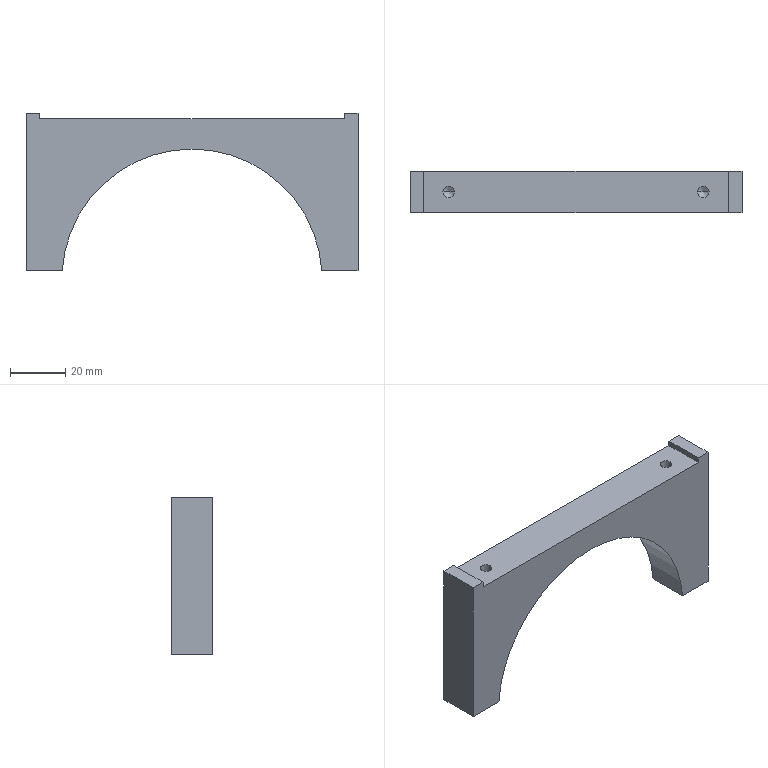Part | STEP file | 11-FG-S01211 | 1 solid | 28 faces | box 120 x 15 x 57 mm | volume 50768 mm3 | plane 11 | cylinder 9 | cone 8 | commonest cylinder face diameters 4.2 x8 94 x1
STEP:
#1=CARTESIAN_POINT('',(-108.1,7.5,42.6));
#2=VERTEX_POINT('',#1);
#3=CARTESIAN_POINT('',(-103.9,7.5,42.6));
#4=VERTEX_POINT('',#3);
#5=CARTESIAN_POINT('',(-106.,7.5,42.6));
#6=DIRECTION('',(0.,0.,1.));
#7=DIRECTION('',(1.,0.,0.));
#8=AXIS2_PLACEMENT_3D('',#5,#6,#7);
#9=CIRCLE('',#8,2.1);
#10=EDGE_CURVE('',#2,#4,#9,.T.);
#11=ORIENTED_EDGE('',*,*,#10,.F.);
#12=CARTESIAN_POINT('',(-108.1,7.5,55.));
#13=VERTEX_POINT('',#12);
#14=CARTESIAN_POINT('',(-108.1,7.5,55.));
#15=DIRECTION('',(0.,0.,1.));
#16=VECTOR('',#15,1000.);
#17=LINE('',#14,#16);
#18=EDGE_CURVE('',#2,#13,#17,.T.);
#19=ORIENTED_EDGE('',*,*,#18,.T.);
#20=CARTESIAN_POINT('',(-103.9,7.5,55.));
#21=VERTEX_POINT('',#20);
#22=CARTESIAN_POINT('',(-106.,7.5,55.));
#23=DIRECTION('',(0.,0.,1.));
#24=DIRECTION('',(1.,0.,0.));
#25=AXIS2_PLACEMENT_3D('',#22,#23,#24);
#26=CIRCLE('',#25,2.1);
#27=EDGE_CURVE('',#13,#21,#26,.T.);
#28=ORIENTED_EDGE('',*,*,#27,.T.);
#29=CARTESIAN_POINT('',(-103.9,7.5,55.));
#30=DIRECTION('',(0.,0.,1.));
#31=VECTOR('',#30,1000.);
#32=LINE('',#29,#31);
#33=EDGE_CURVE('',#4,#21,#32,.T.);
#34=ORIENTED_EDGE('',*,*,#33,.F.);
#35=EDGE_LOOP('',(#11,#19,#28,#34));
#36=FACE_OUTER_BOUND('',#35,.T.);
#37=CARTESIAN_POINT('',(-106.,7.5,55.));
#38=DIRECTION('',(0.,0.,1.));
#39=DIRECTION('',(1.,0.,0.));
#40=AXIS2_PLACEMENT_3D('',#37,#38,#39);
#41=CYLINDRICAL_SURFACE('',#40,2.1);
#42=ADVANCED_FACE('',(#36),#41,.F.);
#43=CARTESIAN_POINT('',(-106.,7.5,41.338));
#44=VERTEX_POINT('',#43);
#45=CARTESIAN_POINT('',(-103.9,7.5,42.6));
#46=DIRECTION('',(0.8572,0.,0.515));
#47=VECTOR('',#46,1000.);
#48=LINE('',#45,#47);
#49=EDGE_CURVE('',#44,#4,#48,.T.);
#50=ORIENTED_EDGE('',*,*,#49,.F.);
#51=CARTESIAN_POINT('',(-108.1,7.5,42.6));
#52=DIRECTION('',(-0.8572,0.,0.515));
#53=VECTOR('',#52,1000.);
#54=LINE('',#51,#53);
#55=EDGE_CURVE('',#44,#2,#54,.T.);
#56=ORIENTED_EDGE('',*,*,#55,.T.);
#57=ORIENTED_EDGE('',*,*,#10,.T.);
#58=EDGE_LOOP('',(#50,#56,#57));
#59=FACE_OUTER_BOUND('',#58,.T.);
#60=CARTESIAN_POINT('',(-106.,7.5,42.6));
#61=DIRECTION('',(0.,0.,1.));
#62=DIRECTION('',(1.,0.,0.));
#63=AXIS2_PLACEMENT_3D('',#60,#61,#62);
#64=CONICAL_SURFACE('',#63,2.1,1.03);
#65=ADVANCED_FACE('',(#59),#64,.F.);
#66=CARTESIAN_POINT('',(-16.1,7.5,42.6));
#67=VERTEX_POINT('',#66);
#68=CARTESIAN_POINT('',(-11.9,7.5,42.6));
#69=VERTEX_POINT('',#68);
#70=CARTESIAN_POINT('',(-14.,7.5,42.6));
#71=DIRECTION('',(0.,0.,1.));
#72=DIRECTION('',(1.,0.,0.));
#73=AXIS2_PLACEMENT_3D('',#70,#71,#72);
#74=CIRCLE('',#73,2.1);
#75=EDGE_CURVE('',#67,#69,#74,.T.);
#76=ORIENTED_EDGE('',*,*,#75,.F.);
#77=CARTESIAN_POINT('',(-16.1,7.5,55.));
#78=VERTEX_POINT('',#77);
#79=CARTESIAN_POINT('',(-16.1,7.5,55.));
#80=DIRECTION('',(0.,0.,1.));
#81=VECTOR('',#80,1000.);
#82=LINE('',#79,#81);
#83=EDGE_CURVE('',#67,#78,#82,.T.);
#84=ORIENTED_EDGE('',*,*,#83,.T.);
#85=CARTESIAN_POINT('',(-11.9,7.5,55.));
#86=VERTEX_POINT('',#85);
#87=CARTESIAN_POINT('',(-14.,7.5,55.));
#88=DIRECTION('',(0.,0.,1.));
#89=DIRECTION('',(1.,0.,0.));
#90=AXIS2_PLACEMENT_3D('',#87,#88,#89);
#91=CIRCLE('',#90,2.1);
#92=EDGE_CURVE('',#78,#86,#91,.T.);
#93=ORIENTED_EDGE('',*,*,#92,.T.);
#94=CARTESIAN_POINT('',(-11.9,7.5,55.));
#95=DIRECTION('',(0.,0.,1.));
#96=VECTOR('',#95,1000.);
#97=LINE('',#94,#96);
#98=EDGE_CURVE('',#69,#86,#97,.T.);
#99=ORIENTED_EDGE('',*,*,#98,.F.);
#100=EDGE_LOOP('',(#76,#84,#93,#99));
#101=FACE_OUTER_BOUND('',#100,.T.);
#102=CARTESIAN_POINT('',(-14.,7.5,55.));
#103=DIRECTION('',(0.,0.,1.));
#104=DIRECTION('',(1.,0.,0.));
#105=AXIS2_PLACEMENT_3D('',#102,#103,#104);
#106=CYLINDRICAL_SURFACE('',#105,2.1);
#107=ADVANCED_FACE('',(#101),#106,.F.);
#108=CARTESIAN_POINT('',(-14.,7.5,41.338));
#109=VERTEX_POINT('',#108);
#110=CARTESIAN_POINT('',(-11.9,7.5,42.6));
#111=DIRECTION('',(0.8572,0.,0.515));
#112=VECTOR('',#111,1000.);
#113=LINE('',#110,#112);
#114=EDGE_CURVE('',#109,#69,#113,.T.);
#115=ORIENTED_EDGE('',*,*,#114,.F.);
#116=CARTESIAN_POINT('',(-16.1,7.5,42.6));
#117=DIRECTION('',(-0.8572,0.,0.515));
#118=VECTOR('',#117,1000.);
#119=LINE('',#116,#118);
#120=EDGE_CURVE('',#109,#67,#119,.T.);
#121=ORIENTED_EDGE('',*,*,#120,.T.);
#122=ORIENTED_EDGE('',*,*,#75,.T.);
#123=EDGE_LOOP('',(#115,#121,#122));
#124=FACE_OUTER_BOUND('',#123,.T.);
#125=CARTESIAN_POINT('',(-14.,7.5,42.6));
#126=DIRECTION('',(0.,0.,1.));
#127=DIRECTION('',(1.,0.,0.));
#128=AXIS2_PLACEMENT_3D('',#125,#126,#127);
#129=CONICAL_SURFACE('',#128,2.1,1.03);
#130=ADVANCED_FACE('',(#124),#129,.F.);
#131=CARTESIAN_POINT('',(-111.4,7.5,12.4));
#132=VERTEX_POINT('',#131);
#133=CARTESIAN_POINT('',(-115.6,7.5,12.4));
#134=VERTEX_POINT('',#133);
#135=CARTESIAN_POINT('',(-113.5,7.5,12.4));
#136=DIRECTION('',(0.,0.,-1.));
#137=DIRECTION('',(-1.,0.,0.));
#138=AXIS2_PLACEMENT_3D('',#135,#136,#137);
#139=CIRCLE('',#138,2.1);
#140=EDGE_CURVE('',#132,#134,#139,.T.);
#141=ORIENTED_EDGE('',*,*,#140,.F.);
#142=CARTESIAN_POINT('',(-111.4,7.5,0.));
#143=VERTEX_POINT('',#142);
#144=CARTESIAN_POINT('',(-111.4,7.5,0.));
#145=DIRECTION('',(0.,0.,-1.));
#146=VECTOR('',#145,1000.);
#147=LINE('',#144,#146);
#148=EDGE_CURVE('',#132,#143,#147,.T.);
#149=ORIENTED_EDGE('',*,*,#148,.T.);
#150=CARTESIAN_POINT('',(-115.6,7.5,0.));
#151=VERTEX_POINT('',#150);
#152=CARTESIAN_POINT('',(-113.5,7.5,0.));
#153=DIRECTION('',(0.,0.,-1.));
#154=DIRECTION('',(-1.,0.,0.));
#155=AXIS2_PLACEMENT_3D('',#152,#153,#154);
#156=CIRCLE('',#155,2.1);
#157=EDGE_CURVE('',#143,#151,#156,.T.);
#158=ORIENTED_EDGE('',*,*,#157,.T.);
#159=CARTESIAN_POINT('',(-115.6,7.5,0.));
#160=DIRECTION('',(0.,0.,-1.));
#161=VECTOR('',#160,1000.);
#162=LINE('',#159,#161);
#163=EDGE_CURVE('',#134,#151,#162,.T.);
#164=ORIENTED_EDGE('',*,*,#163,.F.);
#165=EDGE_LOOP('',(#141,#149,#158,#164));
#166=FACE_OUTER_BOUND('',#165,.T.);
#167=CARTESIAN_POINT('',(-113.5,7.5,0.));
#168=DIRECTION('',(0.,0.,-1.));
#169=DIRECTION('',(-1.,0.,0.));
#170=AXIS2_PLACEMENT_3D('',#167,#168,#169);
#171=CYLINDRICAL_SURFACE('',#170,2.1);
#172=ADVANCED_FACE('',(#166),#171,.F.);
#173=CARTESIAN_POINT('',(-113.5,7.5,13.662));
#174=VERTEX_POINT('',#173);
#175=CARTESIAN_POINT('',(-115.6,7.5,12.4));
#176=DIRECTION('',(-0.8572,0.,-0.515));
#177=VECTOR('',#176,1000.);
#178=LINE('',#175,#177);
#179=EDGE_CURVE('',#174,#134,#178,.T.);
#180=ORIENTED_EDGE('',*,*,#179,.F.);
#181=CARTESIAN_POINT('',(-111.4,7.5,12.4));
#182=DIRECTION('',(0.8572,0.,-0.515));
#183=VECTOR('',#182,1000.);
#184=LINE('',#181,#183);
#185=EDGE_CURVE('',#174,#132,#184,.T.);
#186=ORIENTED_EDGE('',*,*,#185,.T.);
#187=ORIENTED_EDGE('',*,*,#140,.T.);
#188=EDGE_LOOP('',(#180,#186,#187));
#189=FACE_OUTER_BOUND('',#188,.T.);
#190=CARTESIAN_POINT('',(-113.5,7.5,12.4));
#191=DIRECTION('',(0.,0.,-1.));
#192=DIRECTION('',(-1.,0.,0.));
#193=AXIS2_PLACEMENT_3D('',#190,#191,#192);
#194=CONICAL_SURFACE('',#193,2.1,1.03);
#195=ADVANCED_FACE('',(#189),#194,.F.);
#196=CARTESIAN_POINT('',(-4.4,7.5,12.4));
#197=VERTEX_POINT('',#196);
#198=CARTESIAN_POINT('',(-8.6,7.5,12.4));
#199=VERTEX_POINT('',#198);
#200=CARTESIAN_POINT('',(-6.5,7.5,12.4));
#201=DIRECTION('',(0.,0.,-1.));
#202=DIRECTION('',(-1.,0.,0.));
#203=AXIS2_PLACEMENT_3D('',#200,#201,#202);
#204=CIRCLE('',#203,2.1);
#205=EDGE_CURVE('',#197,#199,#204,.T.);
#206=ORIENTED_EDGE('',*,*,#205,.F.);
#207=CARTESIAN_POINT('',(-4.4,7.5,0.));
#208=VERTEX_POINT('',#207);
#209=CARTESIAN_POINT('',(-4.4,7.5,0.));
#210=DIRECTION('',(0.,0.,-1.));
#211=VECTOR('',#210,1000.);
#212=LINE('',#209,#211);
#213=EDGE_CURVE('',#197,#208,#212,.T.);
#214=ORIENTED_EDGE('',*,*,#213,.T.);
#215=CARTESIAN_POINT('',(-8.6,7.5,0.));
#216=VERTEX_POINT('',#215);
#217=CARTESIAN_POINT('',(-6.5,7.5,0.));
#218=DIRECTION('',(0.,0.,-1.));
#219=DIRECTION('',(-1.,0.,0.));
#220=AXIS2_PLACEMENT_3D('',#217,#218,#219);
#221=CIRCLE('',#220,2.1);
#222=EDGE_CURVE('',#208,#216,#221,.T.);
#223=ORIENTED_EDGE('',*,*,#222,.T.);
#224=CARTESIAN_POINT('',(-8.6,7.5,0.));
#225=DIRECTION('',(0.,0.,-1.));
#226=VECTOR('',#225,1000.);
#227=LINE('',#224,#226);
#228=EDGE_CURVE('',#199,#216,#227,.T.);
#229=ORIENTED_EDGE('',*,*,#228,.F.);
#230=EDGE_LOOP('',(#206,#214,#223,#229));
#231=FACE_OUTER_BOUND('',#230,.T.);
#232=CARTESIAN_POINT('',(-6.5,7.5,0.));
#233=DIRECTION('',(0.,0.,-1.));
#234=DIRECTION('',(-1.,0.,0.));
#235=AXIS2_PLACEMENT_3D('',#232,#233,#234);
#236=CYLINDRICAL_SURFACE('',#235,2.1);
#237=ADVANCED_FACE('',(#231),#236,.F.);
#238=CARTESIAN_POINT('',(-6.5,7.5,13.662));
#239=VERTEX_POINT('',#238);
#240=CARTESIAN_POINT('',(-8.6,7.5,12.4));
#241=DIRECTION('',(-0.8572,0.,-0.515));
#242=VECTOR('',#241,1000.);
#243=LINE('',#240,#242);
#244=EDGE_CURVE('',#239,#199,#243,.T.);
#245=ORIENTED_EDGE('',*,*,#244,.F.);
#246=CARTESIAN_POINT('',(-4.4,7.5,12.4));
#247=DIRECTION('',(0.8572,0.,-0.515));
#248=VECTOR('',#247,1000.);
#249=LINE('',#246,#248);
#250=EDGE_CURVE('',#239,#197,#249,.T.);
#251=ORIENTED_EDGE('',*,*,#250,.T.);
#252=ORIENTED_EDGE('',*,*,#205,.T.);
#253=EDGE_LOOP('',(#245,#251,#252));
#254=FACE_OUTER_BOUND('',#253,.T.);
#255=CARTESIAN_POINT('',(-6.5,7.5,12.4));
#256=DIRECTION('',(0.,0.,-1.));
#257=DIRECTION('',(-1.,0.,0.));
#258=AXIS2_PLACEMENT_3D('',#255,#256,#257);
#259=CONICAL_SURFACE('',#258,2.1,1.03);
#260=ADVANCED_FACE('',(#254),#259,.F.);
#261=CARTESIAN_POINT('',(-120.,0.,57.));
#262=VERTEX_POINT('',#261);
#263=CARTESIAN_POINT('',(-115.,0.,57.));
#264=VERTEX_POINT('',#263);
#265=CARTESIAN_POINT('',(-201.,0.,57.));
#266=DIRECTION('',(1.,0.,0.));
#267=VECTOR('',#266,1000.);
#268=LINE('',#265,#267);
#269=EDGE_CURVE('',#262,#264,#268,.T.);
#270=ORIENTED_EDGE('',*,*,#269,.T.);
#271=CARTESIAN_POINT('',(-115.,15.,57.));
#272=VERTEX_POINT('',#271);
#273=CARTESIAN_POINT('',(-115.,15.,57.));
#274=DIRECTION('',(0.,1.,0.));
#275=VECTOR('',#274,1000.);
#276=LINE('',#273,#275);
#277=EDGE_CURVE('',#264,#272,#276,.T.);
#278=ORIENTED_EDGE('',*,*,#277,.T.);
#279=CARTESIAN_POINT('',(-120.,15.,57.));
#280=VERTEX_POINT('',#279);
#281=CARTESIAN_POINT('',(-201.,15.,57.));
#282=DIRECTION('',(1.,0.,0.));
#283=VECTOR('',#282,1000.);
#284=LINE('',#281,#283);
#285=EDGE_CURVE('',#280,#272,#284,.T.);
#286=ORIENTED_EDGE('',*,*,#285,.F.);
#287=CARTESIAN_POINT('',(-120.,0.,57.));
#288=DIRECTION('',(0.,1.,0.));
#289=VECTOR('',#288,1000.);
#290=LINE('',#287,#289);
#291=EDGE_CURVE('',#262,#280,#290,.T.);
#292=ORIENTED_EDGE('',*,*,#291,.F.);
#293=EDGE_LOOP('',(#270,#278,#286,#292));
#294=FACE_OUTER_BOUND('',#293,.T.);
#295=CARTESIAN_POINT('',(-201.,15.,57.));
#296=DIRECTION('',(0.,0.,-1.));
#297=DIRECTION('',(0.,1.,0.));
#298=AXIS2_PLACEMENT_3D('',#295,#296,#297);
#299=PLANE('',#298);
#300=ADVANCED_FACE('',(#294),#299,.F.);
#301=CARTESIAN_POINT('',(-113.5,7.5,0.));
#302=DIRECTION('',(0.,0.,-1.));
#303=DIRECTION('',(-1.,0.,0.));
#304=AXIS2_PLACEMENT_3D('',#301,#302,#303);
#305=CIRCLE('',#304,2.1);
#306=EDGE_CURVE('',#151,#143,#305,.T.);
#307=ORIENTED_EDGE('',*,*,#306,.F.);
#308=ORIENTED_EDGE('',*,*,#157,.F.);
#309=EDGE_LOOP('',(#307,#308));
#310=FACE_BOUND('',#309,.T.);
#311=CARTESIAN_POINT('',(-106.904,15.,0.));
#312=VERTEX_POINT('',#311);
#313=CARTESIAN_POINT('',(-120.,15.,0.));
#314=VERTEX_POINT('',#313);
#315=CARTESIAN_POINT('',(0.,15.,0.));
#316=DIRECTION('',(-1.,0.,0.));
#317=VECTOR('',#316,1000.);
#318=LINE('',#315,#317);
#319=EDGE_CURVE('',#312,#314,#318,.T.);
#320=ORIENTED_EDGE('',*,*,#319,.F.);
#321=CARTESIAN_POINT('',(-106.904,0.,0.));
#322=VERTEX_POINT('',#321);
#323=CARTESIAN_POINT('',(-106.904,80.,0.));
#324=DIRECTION('',(0.,-1.,0.));
#325=VECTOR('',#324,1000.);
#326=LINE('',#323,#325);
#327=EDGE_CURVE('',#312,#322,#326,.T.);
#328=ORIENTED_EDGE('',*,*,#327,.T.);
#329=CARTESIAN_POINT('',(-120.,0.,0.));
#330=VERTEX_POINT('',#329);
#331=CARTESIAN_POINT('',(0.,0.,0.));
#332=DIRECTION('',(1.,0.,0.));
#333=VECTOR('',#332,1000.);
#334=LINE('',#331,#333);
#335=EDGE_CURVE('',#330,#322,#334,.T.);
#336=ORIENTED_EDGE('',*,*,#335,.F.);
#337=CARTESIAN_POINT('',(-120.,0.,0.));
#338=DIRECTION('',(0.,-1.,0.));
#339=VECTOR('',#338,1000.);
#340=LINE('',#337,#339);
#341=EDGE_CURVE('',#314,#330,#340,.T.);
#342=ORIENTED_EDGE('',*,*,#341,.F.);
#343=EDGE_LOOP('',(#320,#328,#336,#342));
#344=FACE_OUTER_BOUND('',#343,.T.);
#345=CARTESIAN_POINT('',(0.,15.,0.));
#346=DIRECTION('',(0.,0.,1.));
#347=DIRECTION('',(1.,0.,0.));
#348=AXIS2_PLACEMENT_3D('',#345,#346,#347);
#349=PLANE('',#348);
#350=ADVANCED_FACE('',(#310,#344),#349,.F.);
#351=CARTESIAN_POINT('',(0.,15.,57.));
#352=VERTEX_POINT('',#351);
#353=CARTESIAN_POINT('',(0.,15.,0.));
#354=VERTEX_POINT('',#353);
#355=CARTESIAN_POINT('',(0.,15.,60.));
#356=DIRECTION('',(0.,0.,-1.));
#357=VECTOR('',#356,1000.);
#358=LINE('',#355,#357);
#359=EDGE_CURVE('',#352,#354,#358,.T.);
#360=ORIENTED_EDGE('',*,*,#359,.F.);
#361=CARTESIAN_POINT('',(0.,0.,57.));
#362=VERTEX_POINT('',#361);
#363=CARTESIAN_POINT('',(0.,15.,57.));
#364=DIRECTION('',(0.,1.,0.));
#365=VECTOR('',#364,1000.);
#366=LINE('',#363,#365);
#367=EDGE_CURVE('',#362,#352,#366,.T.);
#368=ORIENTED_EDGE('',*,*,#367,.F.);
#369=CARTESIAN_POINT('',(0.,0.,0.));
#370=VERTEX_POINT('',#369);
#371=CARTESIAN_POINT('',(0.,0.,60.));
#372=DIRECTION('',(0.,0.,-1.));
#373=VECTOR('',#372,1000.);
#374=LINE('',#371,#373);
#375=EDGE_CURVE('',#362,#370,#374,.T.);
#376=ORIENTED_EDGE('',*,*,#375,.T.);
#377=CARTESIAN_POINT('',(0.,0.,0.));
#378=DIRECTION('',(0.,1.,0.));
#379=VECTOR('',#378,1000.);
#380=LINE('',#377,#379);
#381=EDGE_CURVE('',#370,#354,#380,.T.);
#382=ORIENTED_EDGE('',*,*,#381,.T.);
#383=EDGE_LOOP('',(#360,#368,#376,#382));
#384=FACE_OUTER_BOUND('',#383,.T.);
#385=CARTESIAN_POINT('',(0.,0.,60.));
#386=DIRECTION('',(-1.,0.,0.));
#387=DIRECTION('',(0.,0.,1.));
#388=AXIS2_PLACEMENT_3D('',#385,#386,#387);
#389=PLANE('',#388);
#390=ADVANCED_FACE('',(#384),#389,.F.);
#391=ORIENTED_EDGE('',*,*,#285,.T.);
#392=CARTESIAN_POINT('',(-115.,15.,55.));
#393=VERTEX_POINT('',#392);
#394=CARTESIAN_POINT('',(-115.,15.,57.));
#395=DIRECTION('',(0.,0.,1.));
#396=VECTOR('',#395,1000.);
#397=LINE('',#394,#396);
#398=EDGE_CURVE('',#393,#272,#397,.T.);
#399=ORIENTED_EDGE('',*,*,#398,.F.);
#400=CARTESIAN_POINT('',(-5.,15.,55.));
#401=VERTEX_POINT('',#400);
#402=CARTESIAN_POINT('',(-115.,15.,55.));
#403=DIRECTION('',(-1.,0.,0.));
#404=VECTOR('',#403,1000.);
#405=LINE('',#402,#404);
#406=EDGE_CURVE('',#401,#393,#405,.T.);
#407=ORIENTED_EDGE('',*,*,#406,.F.);
#408=CARTESIAN_POINT('',(-5.,15.,57.));
#409=VERTEX_POINT('',#408);
#410=CARTESIAN_POINT('',(-5.,15.,57.));
#411=DIRECTION('',(0.,0.,-1.));
#412=VECTOR('',#411,1000.);
#413=LINE('',#410,#412);
#414=EDGE_CURVE('',#409,#401,#413,.T.);
#415=ORIENTED_EDGE('',*,*,#414,.F.);
#416=CARTESIAN_POINT('',(-201.,15.,57.));
#417=DIRECTION('',(1.,0.,0.));
#418=VECTOR('',#417,1000.);
#419=LINE('',#416,#418);
#420=EDGE_CURVE('',#409,#352,#419,.T.);
#421=ORIENTED_EDGE('',*,*,#420,.T.);
#422=ORIENTED_EDGE('',*,*,#359,.T.);
#423=CARTESIAN_POINT('',(-13.096,15.,0.));
#424=VERTEX_POINT('',#423);
#425=CARTESIAN_POINT('',(0.,15.,0.));
#426=DIRECTION('',(-1.,0.,0.));
#427=VECTOR('',#426,1000.);
#428=LINE('',#425,#427);
#429=EDGE_CURVE('',#354,#424,#428,.T.);
#430=ORIENTED_EDGE('',*,*,#429,.T.);
#431=CARTESIAN_POINT('',(-60.,15.,-3.));
#432=DIRECTION('',(0.,-1.,0.));
#433=DIRECTION('',(1.,0.,0.));
#434=AXIS2_PLACEMENT_3D('',#431,#432,#433);
#435=CIRCLE('',#434,47.);
#436=EDGE_CURVE('',#424,#312,#435,.T.);
#437=ORIENTED_EDGE('',*,*,#436,.T.);
#438=ORIENTED_EDGE('',*,*,#319,.T.);
#439=CARTESIAN_POINT('',(-120.,15.,60.));
#440=DIRECTION('',(0.,0.,-1.));
#441=VECTOR('',#440,1000.);
#442=LINE('',#439,#441);
#443=EDGE_CURVE('',#280,#314,#442,.T.);
#444=ORIENTED_EDGE('',*,*,#443,.F.);
#445=EDGE_LOOP('',(#391,#399,#407,#415,#421,#422,#430,#437,#438,#444));
#446=FACE_OUTER_BOUND('',#445,.T.);
#447=CARTESIAN_POINT('',(0.,15.,60.));
#448=DIRECTION('',(0.,-1.,0.));
#449=DIRECTION('',(1.,0.,0.));
#450=AXIS2_PLACEMENT_3D('',#447,#448,#449);
#451=PLANE('',#450);
#452=ADVANCED_FACE('',(#446),#451,.F.);
#453=CARTESIAN_POINT('',(-120.,0.,60.));
#454=DIRECTION('',(0.,0.,-1.));
#455=VECTOR('',#454,1000.);
#456=LINE('',#453,#455);
#457=EDGE_CURVE('',#262,#330,#456,.T.);
#458=ORIENTED_EDGE('',*,*,#457,.F.);
#459=ORIENTED_EDGE('',*,*,#291,.T.);
#460=ORIENTED_EDGE('',*,*,#443,.T.);
#461=ORIENTED_EDGE('',*,*,#341,.T.);
#462=EDGE_LOOP('',(#458,#459,#460,#461));
#463=FACE_OUTER_BOUND('',#462,.T.);
#464=CARTESIAN_POINT('',(-120.,0.,60.));
#465=DIRECTION('',(1.,0.,0.));
#466=DIRECTION('',(0.,0.,-1.));
#467=AXIS2_PLACEMENT_3D('',#464,#465,#466);
#468=PLANE('',#467);
#469=ADVANCED_FACE('',(#463),#468,.F.);
#470=CARTESIAN_POINT('',(-5.,0.,55.));
#471=VERTEX_POINT('',#470);
#472=CARTESIAN_POINT('',(-115.,0.,55.));
#473=VERTEX_POINT('',#472);
#474=CARTESIAN_POINT('',(0.,0.,55.));
#475=DIRECTION('',(-1.,0.,0.));
#476=VECTOR('',#475,1000.);
#477=LINE('',#474,#476);
#478=EDGE_CURVE('',#471,#473,#477,.T.);
#479=ORIENTED_EDGE('',*,*,#478,.T.);
#480=CARTESIAN_POINT('',(-115.,0.,60.));
#481=DIRECTION('',(0.,0.,1.));
#482=VECTOR('',#481,1000.);
#483=LINE('',#480,#482);
#484=EDGE_CURVE('',#473,#264,#483,.T.);
#485=ORIENTED_EDGE('',*,*,#484,.T.);
#486=ORIENTED_EDGE('',*,*,#269,.F.);
#487=ORIENTED_EDGE('',*,*,#457,.T.);
#488=ORIENTED_EDGE('',*,*,#335,.T.);
#489=CARTESIAN_POINT('',(-13.096,0.,0.));
#490=VERTEX_POINT('',#489);
#491=CARTESIAN_POINT('',(-60.,0.,-3.));
#492=DIRECTION('',(0.,-1.,0.));
#493=DIRECTION('',(1.,0.,0.));
#494=AXIS2_PLACEMENT_3D('',#491,#492,#493);
#495=CIRCLE('',#494,47.);
#496=EDGE_CURVE('',#490,#322,#495,.T.);
#497=ORIENTED_EDGE('',*,*,#496,.F.);
#498=CARTESIAN_POINT('',(0.,0.,0.));
#499=DIRECTION('',(1.,0.,0.));
#500=VECTOR('',#499,1000.);
#501=LINE('',#498,#500);
#502=EDGE_CURVE('',#490,#370,#501,.T.);
#503=ORIENTED_EDGE('',*,*,#502,.T.);
#504=ORIENTED_EDGE('',*,*,#375,.F.);
#505=CARTESIAN_POINT('',(-5.,0.,57.));
#506=VERTEX_POINT('',#505);
#507=CARTESIAN_POINT('',(-201.,0.,57.));
#508=DIRECTION('',(1.,0.,0.));
#509=VECTOR('',#508,1000.);
#510=LINE('',#507,#509);
#511=EDGE_CURVE('',#506,#362,#510,.T.);
#512=ORIENTED_EDGE('',*,*,#511,.F.);
#513=CARTESIAN_POINT('',(-5.,0.,60.));
#514=DIRECTION('',(0.,0.,-1.));
#515=VECTOR('',#514,1000.);
#516=LINE('',#513,#515);
#517=EDGE_CURVE('',#506,#471,#516,.T.);
#518=ORIENTED_EDGE('',*,*,#517,.T.);
#519=EDGE_LOOP('',(#479,#485,#486,#487,#488,#497,#503,#504,#512,#518));
#520=FACE_OUTER_BOUND('',#519,.T.);
#521=CARTESIAN_POINT('',(0.,0.,60.));
#522=DIRECTION('',(0.,1.,0.));
#523=DIRECTION('',(-1.,0.,0.));
#524=AXIS2_PLACEMENT_3D('',#521,#522,#523);
#525=PLANE('',#524);
#526=ADVANCED_FACE('',(#520),#525,.F.);
#527=CARTESIAN_POINT('',(-6.5,7.5,0.));
#528=DIRECTION('',(0.,0.,-1.));
#529=DIRECTION('',(-1.,0.,0.));
#530=AXIS2_PLACEMENT_3D('',#527,#528,#529);
#531=CIRCLE('',#530,2.1);
#532=EDGE_CURVE('',#216,#208,#531,.T.);
#533=ORIENTED_EDGE('',*,*,#532,.F.);
#534=ORIENTED_EDGE('',*,*,#222,.F.);
#535=EDGE_LOOP('',(#533,#534));
#536=FACE_BOUND('',#535,.T.);
#537=ORIENTED_EDGE('',*,*,#502,.F.);
#538=CARTESIAN_POINT('',(-13.096,80.,0.));
#539=DIRECTION('',(0.,1.,0.));
#540=VECTOR('',#539,1000.);
#541=LINE('',#538,#540);
#542=EDGE_CURVE('',#490,#424,#541,.T.);
#543=ORIENTED_EDGE('',*,*,#542,.T.);
#544=ORIENTED_EDGE('',*,*,#429,.F.);
#545=ORIENTED_EDGE('',*,*,#381,.F.);
#546=EDGE_LOOP('',(#537,#543,#544,#545));
#547=FACE_OUTER_BOUND('',#546,.T.);
#548=CARTESIAN_POINT('',(0.,15.,0.));
#549=DIRECTION('',(0.,0.,1.));
#550=DIRECTION('',(1.,0.,0.));
#551=AXIS2_PLACEMENT_3D('',#548,#549,#550);
#552=PLANE('',#551);
#553=ADVANCED_FACE('',(#536,#547),#552,.F.);
#554=ORIENTED_EDGE('',*,*,#436,.F.);
#555=ORIENTED_EDGE('',*,*,#542,.F.);
#556=ORIENTED_EDGE('',*,*,#496,.T.);
#557=ORIENTED_EDGE('',*,*,#327,.F.);
#558=EDGE_LOOP('',(#554,#555,#556,#557));
#559=FACE_OUTER_BOUND('',#558,.T.);
#560=CARTESIAN_POINT('',(-60.,80.,-3.));
#561=DIRECTION('',(0.,-1.,0.));
#562=DIRECTION('',(1.,0.,0.));
#563=AXIS2_PLACEMENT_3D('',#560,#561,#562);
#564=CYLINDRICAL_SURFACE('',#563,47.);
#565=ADVANCED_FACE('',(#559),#564,.F.);
#566=ORIENTED_EDGE('',*,*,#250,.F.);
#567=ORIENTED_EDGE('',*,*,#244,.T.);
#568=CARTESIAN_POINT('',(-6.5,7.5,12.4));
#569=DIRECTION('',(0.,0.,-1.));
#570=DIRECTION('',(-1.,0.,0.));
#571=AXIS2_PLACEMENT_3D('',#568,#569,#570);
#572=CIRCLE('',#571,2.1);
#573=EDGE_CURVE('',#199,#197,#572,.T.);
#574=ORIENTED_EDGE('',*,*,#573,.T.);
#575=EDGE_LOOP('',(#566,#567,#574));
#576=FACE_OUTER_BOUND('',#575,.T.);
#577=CARTESIAN_POINT('',(-6.5,7.5,12.4));
#578=DIRECTION('',(0.,0.,-1.));
#579=DIRECTION('',(-1.,0.,0.));
#580=AXIS2_PLACEMENT_3D('',#577,#578,#579);
#581=CONICAL_SURFACE('',#580,2.1,1.03);
#582=ADVANCED_FACE('',(#576),#581,.F.);
#583=ORIENTED_EDGE('',*,*,#213,.F.);
#584=ORIENTED_EDGE('',*,*,#573,.F.);
#585=ORIENTED_EDGE('',*,*,#228,.T.);
#586=ORIENTED_EDGE('',*,*,#532,.T.);
#587=EDGE_LOOP('',(#583,#584,#585,#586));
#588=FACE_OUTER_BOUND('',#587,.T.);
#589=CARTESIAN_POINT('',(-6.5,7.5,0.));
#590=DIRECTION('',(0.,0.,-1.));
#591=DIRECTION('',(-1.,0.,0.));
#592=AXIS2_PLACEMENT_3D('',#589,#590,#591);
#593=CYLINDRICAL_SURFACE('',#592,2.1);
#594=ADVANCED_FACE('',(#588),#593,.F.);
#595=ORIENTED_EDGE('',*,*,#185,.F.);
#596=ORIENTED_EDGE('',*,*,#179,.T.);
#597=CARTESIAN_POINT('',(-113.5,7.5,12.4));
#598=DIRECTION('',(0.,0.,-1.));
#599=DIRECTION('',(-1.,0.,0.));
#600=AXIS2_PLACEMENT_3D('',#597,#598,#599);
#601=CIRCLE('',#600,2.1);
#602=EDGE_CURVE('',#134,#132,#601,.T.);
#603=ORIENTED_EDGE('',*,*,#602,.T.);
#604=EDGE_LOOP('',(#595,#596,#603));
#605=FACE_OUTER_BOUND('',#604,.T.);
#606=CARTESIAN_POINT('',(-113.5,7.5,12.4));
#607=DIRECTION('',(0.,0.,-1.));
#608=DIRECTION('',(-1.,0.,0.));
#609=AXIS2_PLACEMENT_3D('',#606,#607,#608);
#610=CONICAL_SURFACE('',#609,2.1,1.03);
#611=ADVANCED_FACE('',(#605),#610,.F.);
#612=ORIENTED_EDGE('',*,*,#148,.F.);
#613=ORIENTED_EDGE('',*,*,#602,.F.);
#614=ORIENTED_EDGE('',*,*,#163,.T.);
#615=ORIENTED_EDGE('',*,*,#306,.T.);
#616=EDGE_LOOP('',(#612,#613,#614,#615));
#617=FACE_OUTER_BOUND('',#616,.T.);
#618=CARTESIAN_POINT('',(-113.5,7.5,0.));
#619=DIRECTION('',(0.,0.,-1.));
#620=DIRECTION('',(-1.,0.,0.));
#621=AXIS2_PLACEMENT_3D('',#618,#619,#620);
#622=CYLINDRICAL_SURFACE('',#621,2.1);
#623=ADVANCED_FACE('',(#617),#622,.F.);
#624=ORIENTED_EDGE('',*,*,#420,.F.);
#625=CARTESIAN_POINT('',(-5.,15.,57.));
#626=DIRECTION('',(0.,-1.,0.));
#627=VECTOR('',#626,1000.);
#628=LINE('',#625,#627);
#629=EDGE_CURVE('',#409,#506,#628,.T.);
#630=ORIENTED_EDGE('',*,*,#629,.T.);
#631=ORIENTED_EDGE('',*,*,#511,.T.);
#632=ORIENTED_EDGE('',*,*,#367,.T.);
#633=EDGE_LOOP('',(#624,#630,#631,#632));
#634=FACE_OUTER_BOUND('',#633,.T.);
#635=CARTESIAN_POINT('',(-201.,15.,57.));
#636=DIRECTION('',(0.,0.,-1.));
#637=DIRECTION('',(0.,1.,0.));
#638=AXIS2_PLACEMENT_3D('',#635,#636,#637);
#639=PLANE('',#638);
#640=ADVANCED_FACE('',(#634),#639,.F.);
#641=CARTESIAN_POINT('',(-106.,7.5,55.));
#642=DIRECTION('',(0.,0.,1.));
#643=DIRECTION('',(1.,0.,0.));
#644=AXIS2_PLACEMENT_3D('',#641,#642,#643);
#645=CIRCLE('',#644,2.1);
#646=EDGE_CURVE('',#21,#13,#645,.T.);
#647=ORIENTED_EDGE('',*,*,#646,.F.);
#648=ORIENTED_EDGE('',*,*,#27,.F.);
#649=EDGE_LOOP('',(#647,#648));
#650=FACE_BOUND('',#649,.T.);
#651=CARTESIAN_POINT('',(-14.,7.5,55.));
#652=DIRECTION('',(0.,0.,1.));
#653=DIRECTION('',(1.,0.,0.));
#654=AXIS2_PLACEMENT_3D('',#651,#652,#653);
#655=CIRCLE('',#654,2.1);
#656=EDGE_CURVE('',#86,#78,#655,.T.);
#657=ORIENTED_EDGE('',*,*,#656,.F.);
#658=ORIENTED_EDGE('',*,*,#92,.F.);
#659=EDGE_LOOP('',(#657,#658));
#660=FACE_BOUND('',#659,.T.);
#661=CARTESIAN_POINT('',(-5.,-186.,55.));
#662=DIRECTION('',(0.,1.,0.));
#663=VECTOR('',#662,1000.);
#664=LINE('',#661,#663);
#665=EDGE_CURVE('',#471,#401,#664,.T.);
#666=ORIENTED_EDGE('',*,*,#665,.T.);
#667=ORIENTED_EDGE('',*,*,#406,.T.);
#668=CARTESIAN_POINT('',(-115.,-186.,55.));
#669=DIRECTION('',(0.,1.,0.));
#670=VECTOR('',#669,1000.);
#671=LINE('',#668,#670);
#672=EDGE_CURVE('',#473,#393,#671,.T.);
#673=ORIENTED_EDGE('',*,*,#672,.F.);
#674=ORIENTED_EDGE('',*,*,#478,.F.);
#675=EDGE_LOOP('',(#666,#667,#673,#674));
#676=FACE_OUTER_BOUND('',#675,.T.);
#677=CARTESIAN_POINT('',(-115.,-186.,55.));
#678=DIRECTION('',(0.,0.,-1.));
#679=DIRECTION('',(-1.,0.,0.));
#680=AXIS2_PLACEMENT_3D('',#677,#678,#679);
#681=PLANE('',#680);
#682=ADVANCED_FACE('',(#650,#660,#676),#681,.F.);
#683=ORIENTED_EDGE('',*,*,#672,.T.);
#684=ORIENTED_EDGE('',*,*,#398,.T.);
#685=ORIENTED_EDGE('',*,*,#277,.F.);
#686=ORIENTED_EDGE('',*,*,#484,.F.);
#687=EDGE_LOOP('',(#683,#684,#685,#686));
#688=FACE_OUTER_BOUND('',#687,.T.);
#689=CARTESIAN_POINT('',(-115.,-186.,57.));
#690=DIRECTION('',(-1.,0.,0.));
#691=DIRECTION('',(0.,-1.,0.));
#692=AXIS2_PLACEMENT_3D('',#689,#690,#691);
#693=PLANE('',#692);
#694=ADVANCED_FACE('',(#688),#693,.F.);
#695=ORIENTED_EDGE('',*,*,#629,.F.);
#696=ORIENTED_EDGE('',*,*,#414,.T.);
#697=ORIENTED_EDGE('',*,*,#665,.F.);
#698=ORIENTED_EDGE('',*,*,#517,.F.);
#699=EDGE_LOOP('',(#695,#696,#697,#698));
#700=FACE_OUTER_BOUND('',#699,.T.);
#701=CARTESIAN_POINT('',(-5.,-186.,57.));
#702=DIRECTION('',(1.,0.,0.));
#703=DIRECTION('',(0.,1.,0.));
#704=AXIS2_PLACEMENT_3D('',#701,#702,#703);
#705=PLANE('',#704);
#706=ADVANCED_FACE('',(#700),#705,.F.);
#707=ORIENTED_EDGE('',*,*,#120,.F.);
#708=ORIENTED_EDGE('',*,*,#114,.T.);
#709=CARTESIAN_POINT('',(-14.,7.5,42.6));
#710=DIRECTION('',(0.,0.,1.));
#711=DIRECTION('',(1.,0.,0.));
#712=AXIS2_PLACEMENT_3D('',#709,#710,#711);
#713=CIRCLE('',#712,2.1);
#714=EDGE_CURVE('',#69,#67,#713,.T.);
#715=ORIENTED_EDGE('',*,*,#714,.T.);
#716=EDGE_LOOP('',(#707,#708,#715));
#717=FACE_OUTER_BOUND('',#716,.T.);
#718=CARTESIAN_POINT('',(-14.,7.5,42.6));
#719=DIRECTION('',(0.,0.,1.));
#720=DIRECTION('',(1.,0.,0.));
#721=AXIS2_PLACEMENT_3D('',#718,#719,#720);
#722=CONICAL_SURFACE('',#721,2.1,1.03);
#723=ADVANCED_FACE('',(#717),#722,.F.);
#724=ORIENTED_EDGE('',*,*,#83,.F.);
#725=ORIENTED_EDGE('',*,*,#714,.F.);
#726=ORIENTED_EDGE('',*,*,#98,.T.);
#727=ORIENTED_EDGE('',*,*,#656,.T.);
#728=EDGE_LOOP('',(#724,#725,#726,#727));
#729=FACE_OUTER_BOUND('',#728,.T.);
#730=CARTESIAN_POINT('',(-14.,7.5,55.));
#731=DIRECTION('',(0.,0.,1.));
#732=DIRECTION('',(1.,0.,0.));
#733=AXIS2_PLACEMENT_3D('',#730,#731,#732);
#734=CYLINDRICAL_SURFACE('',#733,2.1);
#735=ADVANCED_FACE('',(#729),#734,.F.);
#736=ORIENTED_EDGE('',*,*,#55,.F.);
#737=ORIENTED_EDGE('',*,*,#49,.T.);
#738=CARTESIAN_POINT('',(-106.,7.5,42.6));
#739=DIRECTION('',(0.,0.,1.));
#740=DIRECTION('',(1.,0.,0.));
#741=AXIS2_PLACEMENT_3D('',#738,#739,#740);
#742=CIRCLE('',#741,2.1);
#743=EDGE_CURVE('',#4,#2,#742,.T.);
#744=ORIENTED_EDGE('',*,*,#743,.T.);
#745=EDGE_LOOP('',(#736,#737,#744));
#746=FACE_OUTER_BOUND('',#745,.T.);
#747=CARTESIAN_POINT('',(-106.,7.5,42.6));
#748=DIRECTION('',(0.,0.,1.));
#749=DIRECTION('',(1.,0.,0.));
#750=AXIS2_PLACEMENT_3D('',#747,#748,#749);
#751=CONICAL_SURFACE('',#750,2.1,1.03);
#752=ADVANCED_FACE('',(#746),#751,.F.);
#753=ORIENTED_EDGE('',*,*,#18,.F.);
#754=ORIENTED_EDGE('',*,*,#743,.F.);
#755=ORIENTED_EDGE('',*,*,#33,.T.);
#756=ORIENTED_EDGE('',*,*,#646,.T.);
#757=EDGE_LOOP('',(#753,#754,#755,#756));
#758=FACE_OUTER_BOUND('',#757,.T.);
#759=CARTESIAN_POINT('',(-106.,7.5,55.));
#760=DIRECTION('',(0.,0.,1.));
#761=DIRECTION('',(1.,0.,0.));
#762=AXIS2_PLACEMENT_3D('',#759,#760,#761);
#763=CYLINDRICAL_SURFACE('',#762,2.1);
#764=ADVANCED_FACE('',(#758),#763,.F.);
#765=CLOSED_SHELL('',(#42,#65,#107,#130,#172,#195,#237,#260,#300,#350,#390,#452,#469,#526,#553,#565,#582,#594,#611,#623,#640,#682,#694,#706,#723,#735,#752,#764));
#766=MANIFOLD_SOLID_BREP('',#765);
#767=CARTESIAN_POINT('',(0.,0.,0.));
#768=DIRECTION('',(0.,0.,1.));
#769=DIRECTION('',(1.,0.,0.));
#770=AXIS2_PLACEMENT_3D('',#767,#768,#769);
#771=(LENGTH_UNIT()NAMED_UNIT(*)SI_UNIT(.MILLI.,.METRE.));
#772=UNCERTAINTY_MEASURE_WITH_UNIT(LENGTH_MEASURE(0.00001),#771,'','');
#773=(NAMED_UNIT(*)PLANE_ANGLE_UNIT()SI_UNIT($,.RADIAN.));
#774=(NAMED_UNIT(*)SI_UNIT($,.STERADIAN.)SOLID_ANGLE_UNIT());
#775=(GEOMETRIC_REPRESENTATION_CONTEXT(3)GLOBAL_UNCERTAINTY_ASSIGNED_CONTEXT((#772))GLOBAL_UNIT_ASSIGNED_CONTEXT((#771,#773,#774))REPRESENTATION_CONTEXT('',''));
#776=ADVANCED_BREP_SHAPE_REPRESENTATION('',(#766,#770),#775);